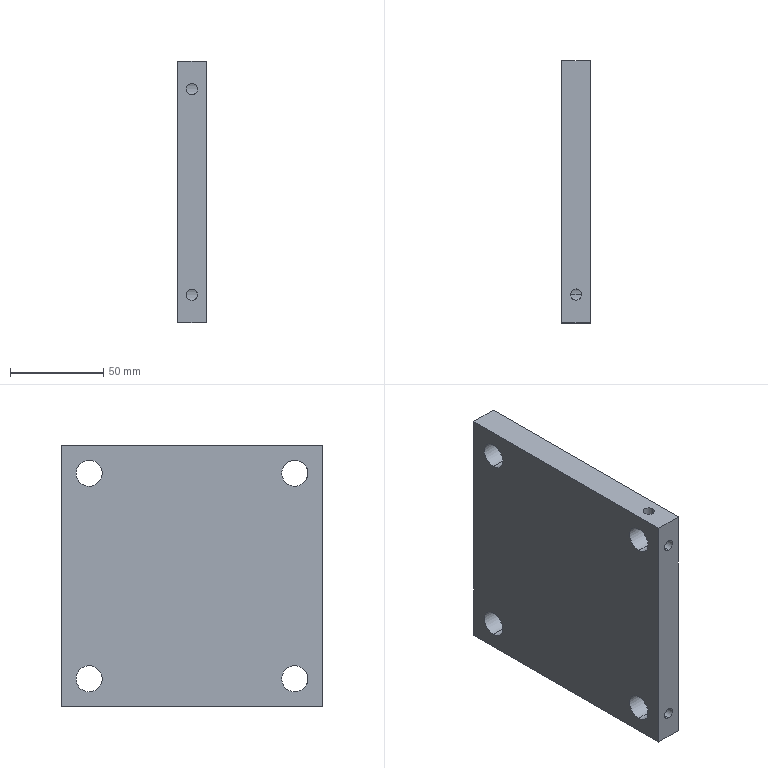Part | STEP file | Positioning_id1566_x_t | 1 solid | 20 faces | box 15 x 140 x 140 mm | volume 284071 mm3 | cylinder 14 | plane 6 | commonest cylinder face diameters 14 x8 6 x6